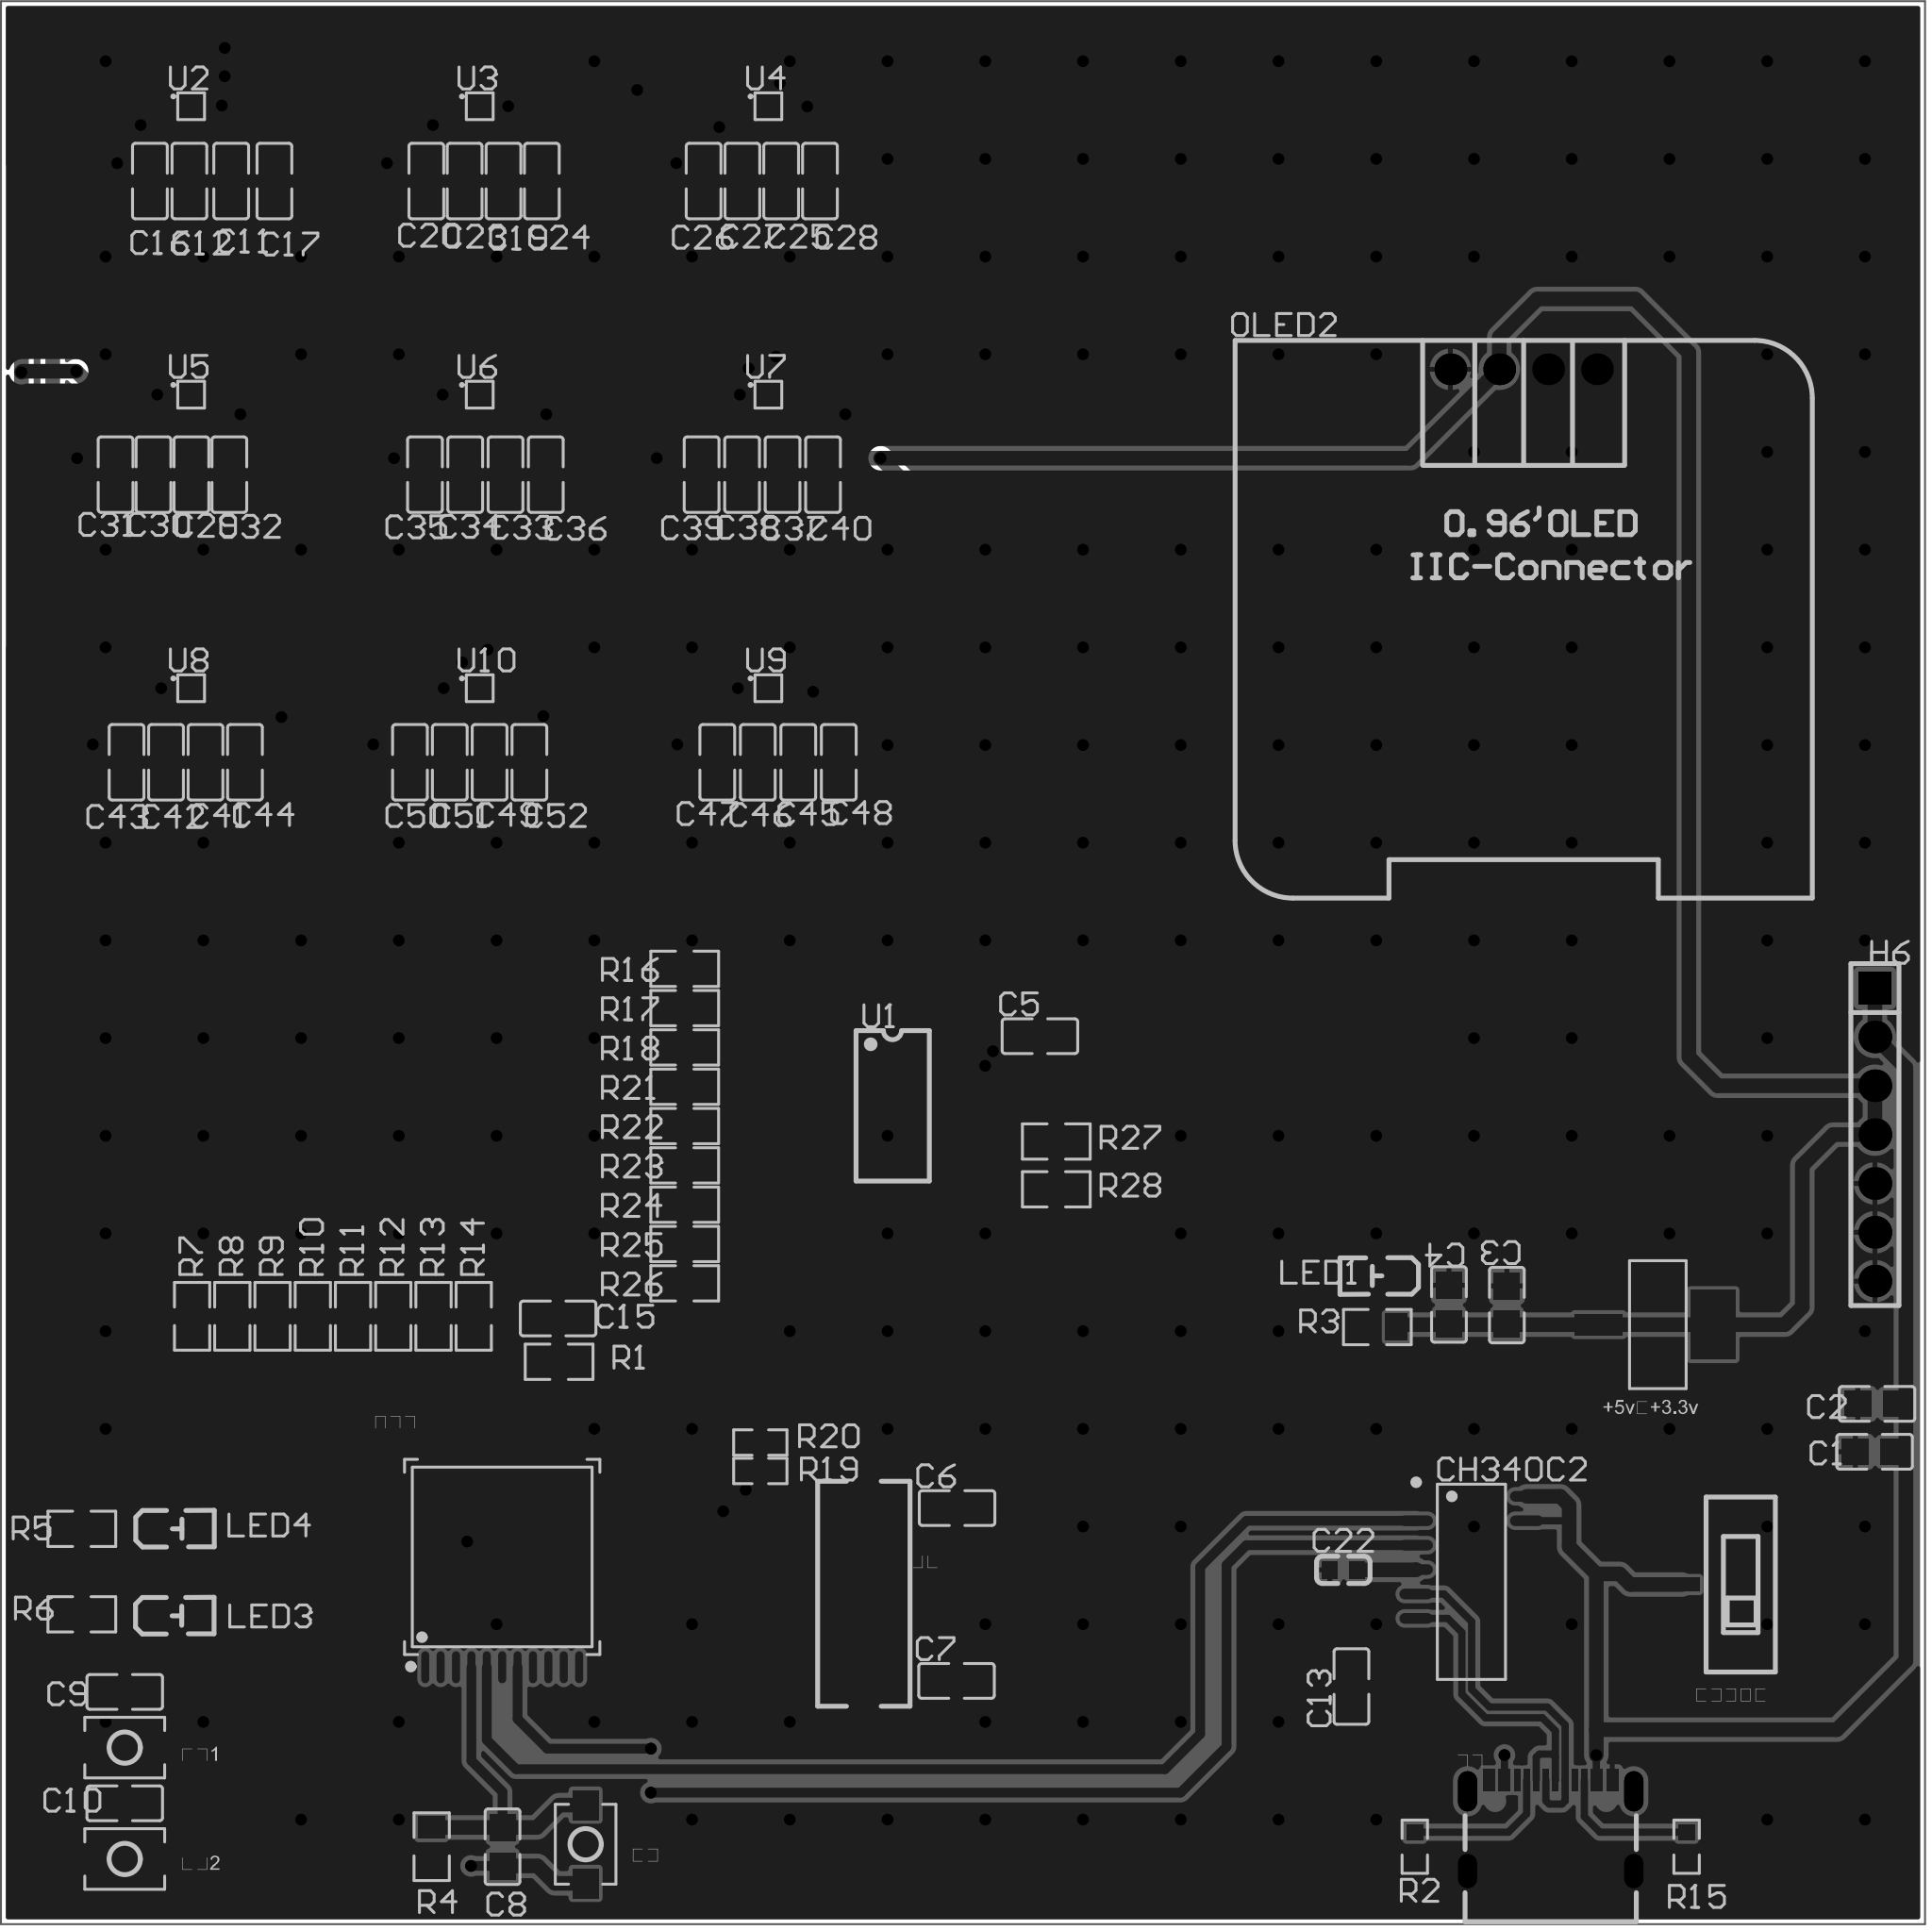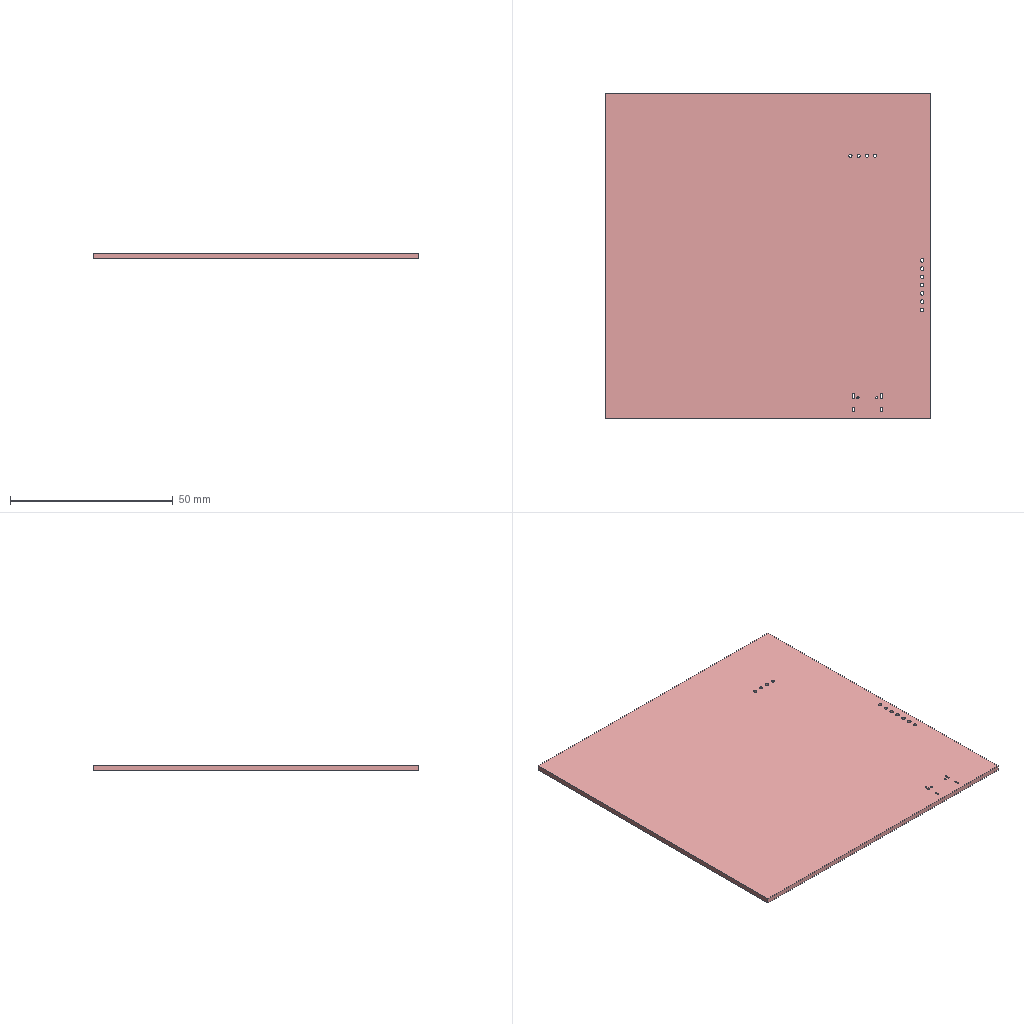Circuit board layout | Altium Designer | box 100 x 100 x 1.6 mm
Layer stack:
# Altium Designer layer stack of  (unit mm; dielectric type: 0 none, 1 core, 2 prepreg, 3 surface material)
index,name,kind,layer,copper_thickness_mm,dielectric_type,dielectric_thickness_mm,dielectric_material,dielectric_constant
0,Top Paste Mask Layer,other,,,,,,
1,Top Silkscreen Layer,other,,,,,,
2,Top Solder Mask Layer,dielectric,,,3,0.01,,3.3
3,Top Layer,copper,Top Layer,0.035,,,,
4,Dielectric1,dielectric,,,3,1.51,FR4,4.5
5,Bottom Layer,copper,Bottom Layer,0.035,,,,
6,Bottom Solder Mask Layer,dielectric,,,3,0.01,,3.3
7,Bottom Silkscreen Layer,other,,,,,,
8,Bottom Paste Mask Layer,other,,,,,,
# drill layer pairs: low layer,high layer
drill_pair,Top Layer,Bottom Layer
Part placement:
Designator,Comment,Layer,Footprint,Center-X(mm),Center-Y(mm),Rotation
C6,22PF,TopLayer,C0805,136.585,111.113,0
C7,22PF,TopLayer,C0805,136.557,102.125,0
晶振,12MHz,TopLayer,CRYSTAL-SMD_L11.4-W4.7-LS12.7,131.739,106.657,270
单片机,STC89C52RC-40I-LQFP44,TopLayer,LQFP-44_L10.0-W10.0-P0.80-LS12.0-BL,112.943,108.571,0
C2,100nF,TopLayer,C0805,184.397,116.532,0
C1,10UF,TopLayer,C0805,184.272,114.041,0
LED1,,TopLayer,LED_0805,158.466,123.184,180
R3,1K,TopLayer,R0805,158.428,120.525,180
C3,100nF,TopLayer,C0805,165.159,121.668,270
C4,10UF,TopLayer,C0805,162.149,121.701,270
+5v转+3.3v,AMS1117-3.3,TopLayer,SOT-223-3_L6.5-W3.4-P2.30-LS7.0-BR,172.906,120.652,180
单片机开关,SS-3235S-L1,TopLayer,SW-SMD_SS-3235S-LX,177.314,107.136,270
H6,,TopLayer,HDR-TH_7P-P2.54-V-M,184.288,130.533,270
R8,10K,TopLayer,R0805,98.918,121.085,90
R13,10K,TopLayer,R0805,109.373,121.085,90
R12,10K,TopLayer,R0805,107.282,121.085,90
R9,10K,TopLayer,R0805,101.009,121.085,90
R11,10K,TopLayer,R0805,105.191,121.085,90
R10,10K,TopLayer,R0805,103.1,121.085,90
R7,10K,TopLayer,R0805,96.827,121.085,90
R14,10K,TopLayer,R0805,111.464,121.085,90
C9,0.1uf,TopLayer,C0805,93.326,101.552,0
功能1,Tact switch 3*4*H,TopLayer,SW-SMD_L4.0-W2.9-LS5.0,93.326,98.656,180
C10,0.1uf,TopLayer,C0805,93.326,95.76,0
功能2,Tact switch 3*4*H,TopLayer,SW-SMD_L4.0-W2.9-LS5.0,93.326,92.864,180
复位,Tact switch 3*4*H,TopLayer,SW-SMD_L4.0-W2.9-LS5.0,117.279,93.631,270
C8,10UF,TopLayer,C0805,112.961,93.504,90
R4,10K,TopLayer,R0805,109.278,93.504,90
LED4,,TopLayer,LED_0805,95.999,110.038,0
LED3,,TopLayer,LED_0805,95.988,105.514,0
R6,1K,TopLayer,R0805,91.096,105.588,180
R5,1K,TopLayer,R0805,91.096,110.033,180
R20,4.7K,TopLayer,R0603,126.358,114.521,180
R19,4.7K,TopLayer,R0603,126.358,113.042,180
C13,0.1UF,TopLayer,C0805,157.08,101.833,90
C22,100nF,TopLayer,C0603,156.658,107.899,0
CH340C2,CH340C,TopLayer,SOP-16_L10.0-W3.9-P1.27-LS6.0-BL,163.317,107.278,270
OLED2,0.96OLED_4P_MODULE_JX,TopLayer,0.96OLED_4P,166.034,170.333,0
C15,0.1uF,TopLayer,C0805,115.85,120.974,180
R1,1K,TopLayer,R0805,115.901,118.72,180
R2,5.1K,TopLayer,R0603,160.373,93.504,90
R15,5.1K,TopLayer,R0603,174.5,93.504,90
电源,Type-C,TopLayer,USB-C-SMD_TYPE-C16PIN,167.437,94.597,0
C5,100nF,TopLayer,C0805,140.891,135.652,0
C11,2.2uF,TopLayer,C0805,98.859,180.121,270
C12,10UF,TopLayer,C0805,96.687,180.121,270
C16,0.1UF,TopLayer,C0805,94.634,180.121,90
C17,0.1UF,TopLayer,C0805,101.105,180.121,90
C19,2.2uF,TopLayer,C0805,113.01,180.121,270
C20,10UF,TopLayer,C0805,109.002,180.121,270
C23,0.1UF,TopLayer,C0805,110.991,180.121,90
C24,0.1UF,TopLayer,C0805,115.003,180.121,90
C25,2.2uF,TopLayer,C0805,127.442,180.121,270
C26,10UF,TopLayer,C0805,123.411,180.121,270
C27,0.1UF,TopLayer,C0805,125.427,180.121,90
C28,0.1UF,TopLayer,C0805,129.458,180.121,90
C29,2.2uF,TopLayer,C0805,96.792,164.853,270
C30,10UF,TopLayer,C0805,94.82,164.853,270
C31,0.1UF,TopLayer,C0805,92.849,164.853,90
C32,0.1UF,TopLayer,C0805,98.763,164.853,90
C33,2.2uF,TopLayer,C0805,113.116,164.853,270
C34,10UF,TopLayer,C0805,111.023,164.853,270
C35,0.1UF,TopLayer,C0805,108.93,164.853,90
C36,0.1UF,TopLayer,C0805,115.209,164.853,90
C37,2.2uF,TopLayer,C0805,127.514,164.853,270
C38,10UF,TopLayer,C0805,125.41,164.853,270
C39,0.1UF,TopLayer,C0805,123.307,164.853,90
C40,0.1UF,TopLayer,C0805,129.618,164.853,90
C41,2.2uF,TopLayer,C0805,97.523,149.896,270
C42,10UF,TopLayer,C0805,95.472,149.896,270
C43,0.1UF,TopLayer,C0805,93.421,149.896,90
C44,0.1UF,TopLayer,C0805,99.574,149.896,90
C45,2.2uF,TopLayer,C0805,128.332,149.896,270
C46,10UF,TopLayer,C0805,126.227,149.896,270
C47,0.1UF,TopLayer,C0805,124.123,149.896,90
C48,0.1UF,TopLayer,C0805,130.436,149.896,90
C49,2.2uF,TopLayer,C0805,112.288,149.896,270
C50,10UF,TopLayer,C0805,108.15,149.896,270
C51,0.1UF,TopLayer,C0805,110.219,149.896,90
C52,0.1UF,TopLayer,C0805,114.358,149.896,90
R16,10K,TopLayer,R0805,122.429,139.156,0
R17,4.7K,TopLayer,R0805,122.429,137.112,0
R18,4.7K,TopLayer,R0805,122.429,135.067,0
R21,4.7K,TopLayer,R0805,122.429,133.023,0
R22,4.7K,TopLayer,R0805,122.429,130.978,0
R23,4.7K,TopLayer,R0805,122.429,128.934,0
R24,4.7K,TopLayer,R0805,122.429,126.889,0
R25,4.7K,TopLayer,R0805,122.429,124.845,0
R26,4.7K,TopLayer,R0805,122.429,122.8,0
R27,4.7K,TopLayer,R0805,141.743,130.175,0
R28,4.7K,TopLayer,R0805,141.743,127.689,0
U1,TCA9548APWR,TopLayer,TSSOP-24_L7.8-W4.4-P0.65-LS6.4-BL,133.239,132.056,270
U2,BMM350,TopLayer,WLCSP-9_L1.3-W1.3-R3-C3-P0.40-TL,96.776,184.012,0
U3,BMM350,TopLayer,WLCSP-9_L1.3-W1.3-R3-C3-P0.40-TL,111.776,184.012,0
U4,BMM350,TopLayer,WLCSP-9_L1.3-W1.3-R3-C3-P0.40-TL,126.777,184.012,0
U5,BMM350,TopLayer,WLCSP-9_L1.3-W1.3-R3-C3-P0.40-TL,96.776,169.012,0
U6,BMM350,TopLayer,WLCSP-9_L1.3-W1.3-R3-C3-P0.40-TL,111.776,169.012,0
U7,BMM350,TopLayer,WLCSP-9_L1.3-W1.3-R3-C3-P0.40-TL,126.777,169.012,0
U8,BMM350,TopLayer,WLCSP-9_L1.3-W1.3-R3-C3-P0.40-TL,96.776,153.748,0
U9,BMM350,TopLayer,WLCSP-9_L1.3-W1.3-R3-C3-P0.40-TL,126.777,153.748,0
U10,BMM350,TopLayer,WLCSP-9_L1.3-W1.3-R3-C3-P0.40-TL,111.776,153.748,0
Pad and via stacks:
# Altium Designer via and pad stacks of  (unit mm). Each distinct definition once, with the count of objects using it.
# via: kind,start_layer,end_layer,hole_mm,diameter_mm,mode(0 simple;1 top-mid-bottom;2 full stack),diameter_per_layer,count,example_net
# pad: kind,layer,hole_mm,hole_type(0 round;1 square;2 slot),plating,top_size,top_shape(1 round;2 rect;3 octagon;9 rounded rect),mid_size,bottom_size,mode,footprint,size_per_layer,count,example
pad,Top Layer,0,0,plated,1.41x1.35,2,1.41x1.35,1.41x1.35,0,C0805,,96,C6.2
pad,Top Layer,0,0,plated,5.5x1.4,2,5.5x1.4,5.5x1.4,0,CRYSTAL-SMD_L11.4-W4.7-LS12.7,,2,\u6676\u632F.2
pad,Top Layer,0,0,plated,0.42x1.67,1,0.42x1.67,0.42x1.67,0,LQFP-44_L10.0-W10.0-P0.80-LS12.0-BL,,22,\u5355\u7247\u673A.1
pad,Top Layer,0,0,plated,1.67x0.42,1,1.67x0.42,1.67x0.42,0,LQFP-44_L10.0-W10.0-P0.80-LS12.0-BL,,22,\u5355\u7247\u673A.12
pad,Top Layer,0,0,plated,1x1.25,2,1x1.25,1x1.25,0,LED_0805,,6,LED1.2
pad,Top Layer,0,0,plated,1.133x1.377,2,1.133x1.377,1.133x1.377,0,R0805,,48,R3.2
pad,Top Layer,0,0,plated,2.5x1.1,2,2.5x1.1,2.5x1.1,0,SOT-223-3_L6.5-W3.4-P2.30-LS7.0-BR,,3,+5v\u8F6C+3.3v.1
pad,Top Layer,0,0,plated,2.34x3.6,2,2.34x3.6,2.34x3.6,0,SOT-223-3_L6.5-W3.4-P2.30-LS7.0-BR,,1,+5v\u8F6C+3.3v.4
pad,Top Layer,0,0,plated,0.7x1.8,2,0.7x1.8,0.7x1.8,0,SW-SMD_SS-3235S-LX,,6,\u5355\u7247\u673A\u5F00\u5173.1
pad,Top Layer,0,0,plated,1.53x1.36,2,1.53x1.36,1.53x1.36,0,SW-SMD_L4.0-W2.9-LS5.0,,6,\u529F\u80FD1.1
pad,Top Layer,0,0,plated,0.8065x0.864,2,0.8065x0.864,0.8065x0.864,0,R0603,,8,R20.2
pad,Top Layer,0,0,plated,0.8x0.9,2,0.8x0.9,0.8x0.9,0,C0603,,2,C22.2
pad,Top Layer,0,0,plated,0.56x1.745,1,0.56x1.745,0.56x1.745,0,SOP-16_L10.0-W3.9-P1.27-LS6.0-BL,,16,CH340C2.1
pad,Top Layer,0,0,plated,0.6x1.15,2,0.6x1.15,0.6x1.15,0,USB-C-SMD_TYPE-C16PIN,,4,\u7535\u6E90.A1B12
pad,Top Layer,0,0,plated,0.3x1.15,2,0.3x1.15,0.3x1.15,0,USB-C-SMD_TYPE-C16PIN,,8,\u7535\u6E90.B5
pad,Top Layer,0,0,plated,0.4x1.65,2,0.4x1.65,0.4x1.65,0,TSSOP-24_L7.8-W4.4-P0.65-LS6.4-BL,,24,U1.6
pad,Top Layer,0,0,plated,0.2x0.2,1,0.2x0.2,0.2x0.2,0,WLCSP-9_L1.3-W1.3-R3-C3-P0.40-TL,,81,U2.A1
pad,Multi-Layer,1.1,0,plated,1.7x1.7,2,1.7x1.7,1.7x1.7,0,HDR-TH_7P-P2.54-V-M,,1,H6.1
pad,Multi-Layer,1.1,0,plated,1.7x1.7,1,1.7x1.7,1.7x1.7,0,HDR-TH_7P-P2.54-V-M,,6,H6.2
pad,Multi-Layer,1,0,plated,1.65x1.65,1,1.65x1.65,1.65x1.65,0,0.96OLED_4P,,4,OLED2.4
pad,Multi-Layer,0.6,2,plated,1x1.8,1,1x1.8,1x1.8,0,USB-C-SMD_TYPE-C16PIN,,2,\u7535\u6E90.4
pad,Multi-Layer,0.6,2,plated,1x2.1,1,1x2.1,1x2.1,0,USB-C-SMD_TYPE-C16PIN,,2,\u7535\u6E90.2
via,Top Layer,Bottom Layer,0.3048,0.61,0,,280,$1N4040
Copper pours:
name,layer,net,type(0 solid;1 hatched;2 none)
Bottom Layer-GND,Bottom Layer,GND,0
Top Layer-GND,Top Layer,GND,0